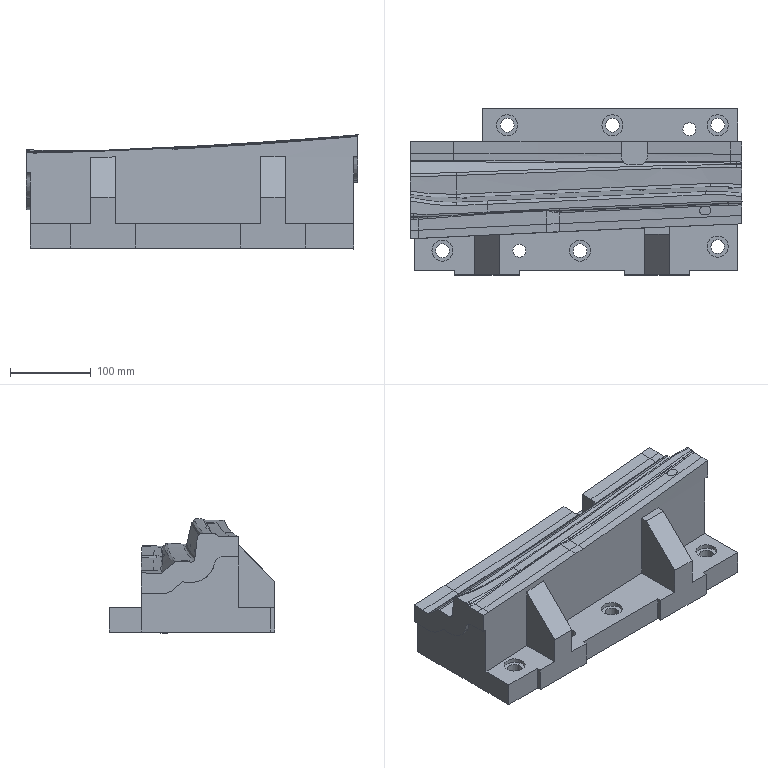Part | NX | features solid 2 | 1 solid | 123 faces | box 410.693 x 205 x 139.836 mm | volume 5811322 mm3 | spline 72 | plane 35 | cylinder 16 | commonest cylinder face diameters 17 x6 26 x6 16 x2 20 x2